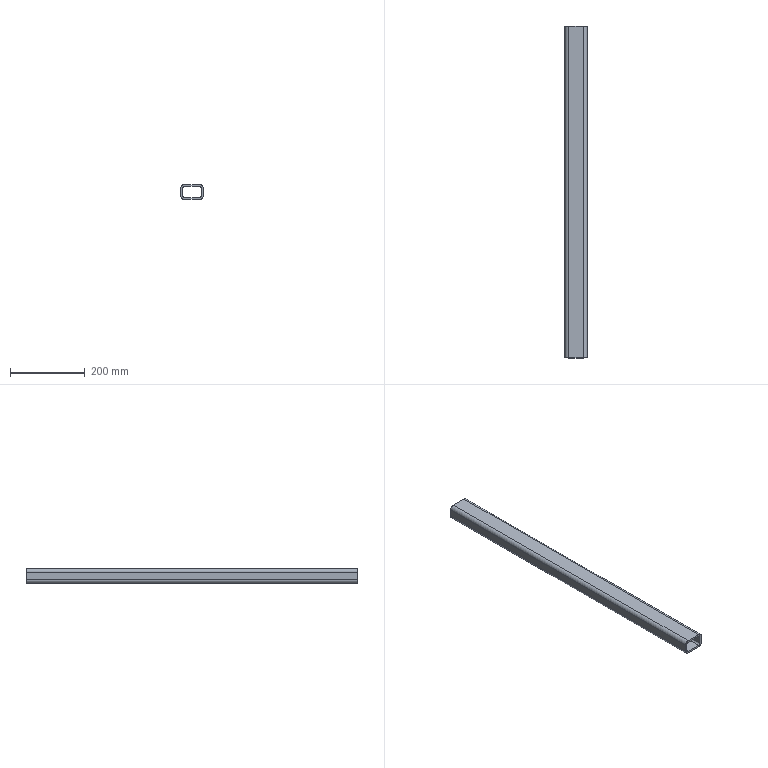Part | STEP file | body floor crossmember--000.001--20240926 | 1 solid | 18 faces | box 60 x 887 x 40 mm | volume 741194 mm3 | plane 10 | cylinder 8 | commonest cylinder face diameters 10 x4 20 x4